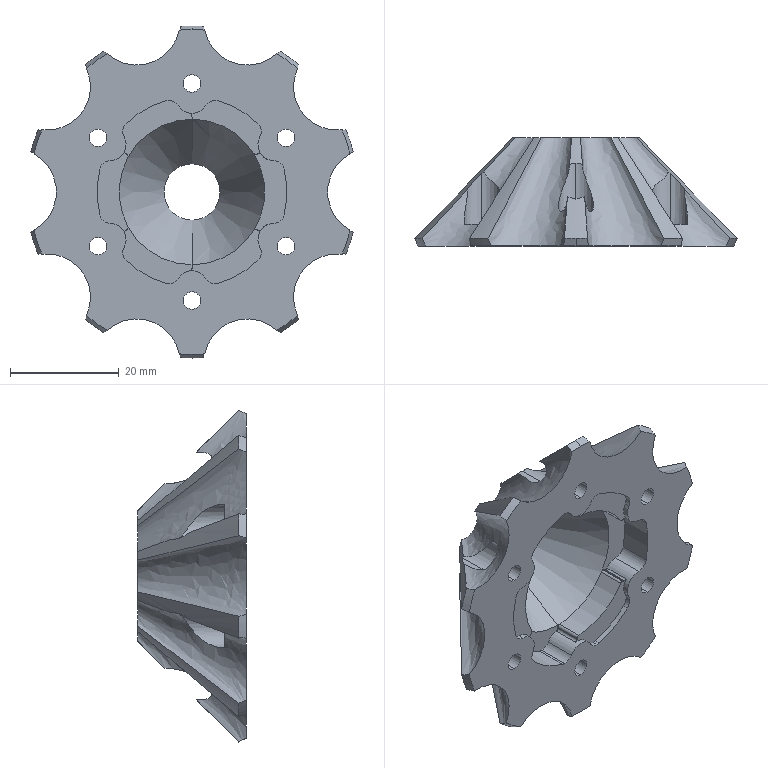Part | SolidWorks | features ICE 6, Blend 2, Chamfer 2, Fillet 2, BlendCut 1, Revolution 1 | 1 solid | 131 faces | box 59.347 x 20 x 61.172 mm | volume 14853 mm3 | cylinder 72 | cone 29 | plane 20 | spline 10 | commonest cylinder face diameters 6.5 x16 1 x14 4 x14 3.2 x12 6 x7 35 x6